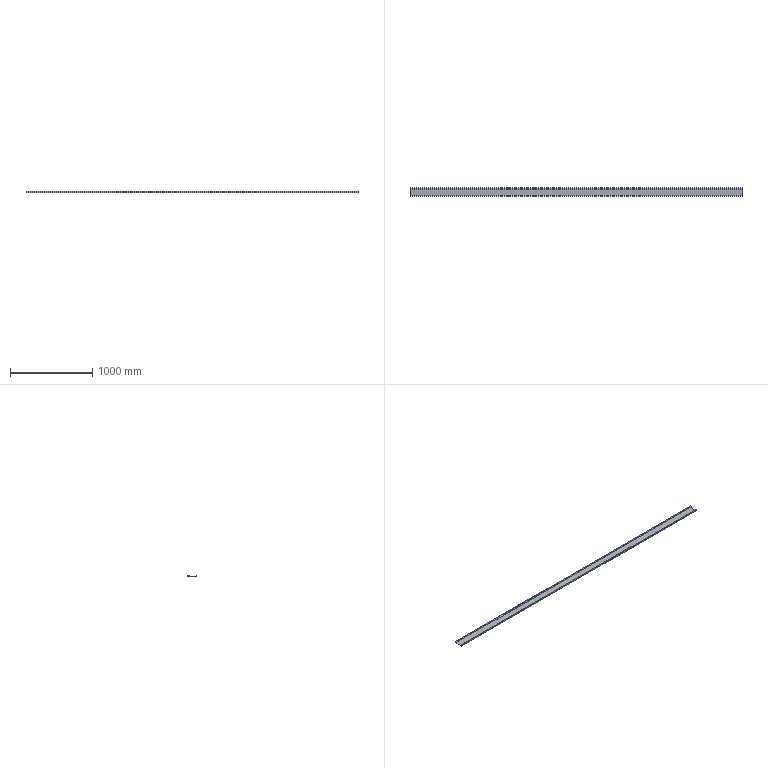Part | STEP file | E3-Electrical cabinet guardrail 1 toe plate | 1 solid | 18 faces | box 4025 x 100 x 20 mm | volume 925227 mm3 | plane 12 | cylinder 6 | commonest cylinder face diameters 2 x3 5 x3
STEP:
#1=CARTESIAN_POINT('',(0.,0.,0.));
#2=DIRECTION('',(0.,0.,1.));
#3=DIRECTION('',(1.,0.,0.));
#4=AXIS2_PLACEMENT_3D('',#1,#2,#3);
#5=CARTESIAN_POINT('',(-2012.5,1.5,2.5));
#6=VERTEX_POINT('',#5);
#7=CARTESIAN_POINT('',(-2012.5,1.5,20.));
#8=VERTEX_POINT('',#7);
#9=CARTESIAN_POINT('',(-2012.5,1.5,2.5));
#10=DIRECTION('',(0.,0.,1.));
#11=VECTOR('',#10,1.);
#12=LINE('',#9,#11);
#13=CARTESIAN_POINT('',(2012.5,1.5,2.5));
#14=DIRECTION('',(0.,-1.,0.));
#15=DIRECTION('',(0.,0.,-1.));
#16=AXIS2_PLACEMENT_3D('',#13,#14,#15);
#17=PLANE('',#16);
#18=CARTESIAN_POINT('',(0.,-4025.));
#19=DIRECTION('',(-1.,0.));
#20=VECTOR('',#19,1.);
#21=LINE('',#18,#20);
#22=(GEOMETRIC_REPRESENTATION_CONTEXT(2)PARAMETRIC_REPRESENTATION_CONTEXT()REPRESENTATION_CONTEXT('',''));
#23=DEFINITIONAL_REPRESENTATION('',(#21),#22);
#24=PCURVE('',#17,#23);
#25=CARTESIAN_POINT('',(-2012.5,2.5,2.5));
#26=DIRECTION('',(-1.,0.,0.));
#27=DIRECTION('',(0.,0.,1.));
#28=AXIS2_PLACEMENT_3D('',#25,#26,#27);
#29=PLANE('',#28);
#30=CARTESIAN_POINT('',(0.,-1.));
#31=DIRECTION('',(1.,0.));
#32=VECTOR('',#31,1.);
#33=LINE('',#30,#32);
#34=(GEOMETRIC_REPRESENTATION_CONTEXT(2)PARAMETRIC_REPRESENTATION_CONTEXT()REPRESENTATION_CONTEXT('',''));
#35=DEFINITIONAL_REPRESENTATION('',(#33),#34);
#36=PCURVE('',#29,#35);
#37=SURFACE_CURVE('',#12,(#24,#36),.PCURVE_S1.);
#38=EDGE_CURVE('',#6,#8,#37,.T.);
#39=ORIENTED_EDGE('',*,*,#38,.T.);
#40=CARTESIAN_POINT('',(2012.5,1.5,20.));
#41=VERTEX_POINT('',#40);
#42=CARTESIAN_POINT('',(2012.5,1.5,20.));
#43=DIRECTION('',(-1.,0.,0.));
#44=VECTOR('',#43,1.);
#45=LINE('',#42,#44);
#46=CARTESIAN_POINT('',(-17.5,0.));
#47=DIRECTION('',(0.,-1.));
#48=VECTOR('',#47,1.);
#49=LINE('',#46,#48);
#50=(GEOMETRIC_REPRESENTATION_CONTEXT(2)PARAMETRIC_REPRESENTATION_CONTEXT()REPRESENTATION_CONTEXT('',''));
#51=DEFINITIONAL_REPRESENTATION('',(#49),#50);
#52=PCURVE('',#17,#51);
#53=CARTESIAN_POINT('',(2012.5,0.,20.));
#54=DIRECTION('',(0.,0.,1.));
#55=DIRECTION('',(1.,0.,0.));
#56=AXIS2_PLACEMENT_3D('',#53,#54,#55);
#57=PLANE('',#56);
#58=CARTESIAN_POINT('',(0.,1.5));
#59=DIRECTION('',(-1.,0.));
#60=VECTOR('',#59,1.);
#61=LINE('',#58,#60);
#62=(GEOMETRIC_REPRESENTATION_CONTEXT(2)PARAMETRIC_REPRESENTATION_CONTEXT()REPRESENTATION_CONTEXT('',''));
#63=DEFINITIONAL_REPRESENTATION('',(#61),#62);
#64=PCURVE('',#57,#63);
#65=SURFACE_CURVE('',#45,(#52,#64),.PCURVE_S1.);
#66=EDGE_CURVE('',#41,#8,#65,.T.);
#67=ORIENTED_EDGE('',*,*,#66,.F.);
#68=CARTESIAN_POINT('',(2012.5,1.5,2.5));
#69=VERTEX_POINT('',#68);
#70=CARTESIAN_POINT('',(2012.5,1.5,2.5));
#71=DIRECTION('',(0.,0.,1.));
#72=VECTOR('',#71,1.);
#73=LINE('',#70,#72);
#74=CARTESIAN_POINT('',(0.,0.));
#75=DIRECTION('',(-1.,0.));
#76=VECTOR('',#75,1.);
#77=LINE('',#74,#76);
#78=(GEOMETRIC_REPRESENTATION_CONTEXT(2)PARAMETRIC_REPRESENTATION_CONTEXT()REPRESENTATION_CONTEXT('',''));
#79=DEFINITIONAL_REPRESENTATION('',(#77),#78);
#80=PCURVE('',#17,#79);
#81=CARTESIAN_POINT('',(2012.5,2.5,2.5));
#82=DIRECTION('',(-1.,0.,0.));
#83=DIRECTION('',(0.,0.,1.));
#84=AXIS2_PLACEMENT_3D('',#81,#82,#83);
#85=PLANE('',#84);
#86=CARTESIAN_POINT('',(0.,-1.));
#87=DIRECTION('',(1.,0.));
#88=VECTOR('',#87,1.);
#89=LINE('',#86,#88);
#90=(GEOMETRIC_REPRESENTATION_CONTEXT(2)PARAMETRIC_REPRESENTATION_CONTEXT()REPRESENTATION_CONTEXT('',''));
#91=DEFINITIONAL_REPRESENTATION('',(#89),#90);
#92=PCURVE('',#85,#91);
#93=SURFACE_CURVE('',#73,(#80,#92),.PCURVE_S1.);
#94=EDGE_CURVE('',#69,#41,#93,.T.);
#95=ORIENTED_EDGE('',*,*,#94,.F.);
#96=CARTESIAN_POINT('',(2012.5,1.5,2.5));
#97=DIRECTION('',(-1.,0.,0.));
#98=VECTOR('',#97,1.);
#99=LINE('',#96,#98);
#100=CARTESIAN_POINT('',(0.,0.));
#101=DIRECTION('',(0.,-1.));
#102=VECTOR('',#101,1.);
#103=LINE('',#100,#102);
#104=(GEOMETRIC_REPRESENTATION_CONTEXT(2)PARAMETRIC_REPRESENTATION_CONTEXT()REPRESENTATION_CONTEXT('',''));
#105=DEFINITIONAL_REPRESENTATION('',(#103),#104);
#106=PCURVE('',#17,#105);
#107=CARTESIAN_POINT('',(2012.5,2.5,2.5));
#108=DIRECTION('',(-1.,0.,0.));
#109=DIRECTION('',(0.,0.,1.));
#110=AXIS2_PLACEMENT_3D('',#107,#108,#109);
#111=CYLINDRICAL_SURFACE('',#110,1.);
#112=CARTESIAN_POINT('',(4.712,0.));
#113=DIRECTION('',(0.,1.));
#114=VECTOR('',#113,1.);
#115=LINE('',#112,#114);
#116=(GEOMETRIC_REPRESENTATION_CONTEXT(2)PARAMETRIC_REPRESENTATION_CONTEXT()REPRESENTATION_CONTEXT('',''));
#117=DEFINITIONAL_REPRESENTATION('',(#115),#116);
#118=PCURVE('',#111,#117);
#119=SURFACE_CURVE('',#99,(#106,#118),.PCURVE_S1.);
#120=EDGE_CURVE('',#69,#6,#119,.T.);
#121=ORIENTED_EDGE('',*,*,#120,.T.);
#122=EDGE_LOOP('',(#39,#67,#95,#121));
#123=FACE_BOUND('',#122,.T.);
#124=ADVANCED_FACE('',(#123),#17,.F.);
#125=CARTESIAN_POINT('',(-2012.5,0.,20.));
#126=VERTEX_POINT('',#125);
#127=CARTESIAN_POINT('',(-2012.5,0.,20.));
#128=DIRECTION('',(0.,1.,0.));
#129=VECTOR('',#128,1.);
#130=LINE('',#127,#129);
#131=CARTESIAN_POINT('',(-4025.,0.));
#132=DIRECTION('',(0.,1.));
#133=VECTOR('',#132,1.);
#134=LINE('',#131,#133);
#135=(GEOMETRIC_REPRESENTATION_CONTEXT(2)PARAMETRIC_REPRESENTATION_CONTEXT()REPRESENTATION_CONTEXT('',''));
#136=DEFINITIONAL_REPRESENTATION('',(#134),#135);
#137=PCURVE('',#57,#136);
#138=CARTESIAN_POINT('',(17.5,-2.5));
#139=DIRECTION('',(0.,1.));
#140=VECTOR('',#139,1.);
#141=LINE('',#138,#140);
#142=(GEOMETRIC_REPRESENTATION_CONTEXT(2)PARAMETRIC_REPRESENTATION_CONTEXT()REPRESENTATION_CONTEXT('',''));
#143=DEFINITIONAL_REPRESENTATION('',(#141),#142);
#144=PCURVE('',#29,#143);
#145=SURFACE_CURVE('',#130,(#137,#144),.PCURVE_S1.);
#146=EDGE_CURVE('',#126,#8,#145,.T.);
#147=ORIENTED_EDGE('',*,*,#146,.F.);
#148=CARTESIAN_POINT('',(2012.5,0.,20.));
#149=VERTEX_POINT('',#148);
#150=CARTESIAN_POINT('',(2012.5,0.,20.));
#151=DIRECTION('',(-1.,0.,0.));
#152=VECTOR('',#151,1.);
#153=LINE('',#150,#152);
#154=CARTESIAN_POINT('',(0.,0.));
#155=DIRECTION('',(-1.,0.));
#156=VECTOR('',#155,1.);
#157=LINE('',#154,#156);
#158=(GEOMETRIC_REPRESENTATION_CONTEXT(2)PARAMETRIC_REPRESENTATION_CONTEXT()REPRESENTATION_CONTEXT('',''));
#159=DEFINITIONAL_REPRESENTATION('',(#157),#158);
#160=PCURVE('',#57,#159);
#161=CARTESIAN_POINT('',(2012.5,0.,2.5));
#162=DIRECTION('',(0.,-1.,0.));
#163=DIRECTION('',(0.,0.,-1.));
#164=AXIS2_PLACEMENT_3D('',#161,#162,#163);
#165=PLANE('',#164);
#166=CARTESIAN_POINT('',(-17.5,0.));
#167=DIRECTION('',(0.,-1.));
#168=VECTOR('',#167,1.);
#169=LINE('',#166,#168);
#170=(GEOMETRIC_REPRESENTATION_CONTEXT(2)PARAMETRIC_REPRESENTATION_CONTEXT()REPRESENTATION_CONTEXT('',''));
#171=DEFINITIONAL_REPRESENTATION('',(#169),#170);
#172=PCURVE('',#165,#171);
#173=SURFACE_CURVE('',#153,(#160,#172),.PCURVE_S1.);
#174=EDGE_CURVE('',#149,#126,#173,.T.);
#175=ORIENTED_EDGE('',*,*,#174,.F.);
#176=CARTESIAN_POINT('',(2012.5,0.,20.));
#177=DIRECTION('',(0.,1.,0.));
#178=VECTOR('',#177,1.);
#179=LINE('',#176,#178);
#180=CARTESIAN_POINT('',(0.,0.));
#181=DIRECTION('',(0.,1.));
#182=VECTOR('',#181,1.);
#183=LINE('',#180,#182);
#184=(GEOMETRIC_REPRESENTATION_CONTEXT(2)PARAMETRIC_REPRESENTATION_CONTEXT()REPRESENTATION_CONTEXT('',''));
#185=DEFINITIONAL_REPRESENTATION('',(#183),#184);
#186=PCURVE('',#57,#185);
#187=CARTESIAN_POINT('',(17.5,-2.5));
#188=DIRECTION('',(0.,1.));
#189=VECTOR('',#188,1.);
#190=LINE('',#187,#189);
#191=(GEOMETRIC_REPRESENTATION_CONTEXT(2)PARAMETRIC_REPRESENTATION_CONTEXT()REPRESENTATION_CONTEXT('',''));
#192=DEFINITIONAL_REPRESENTATION('',(#190),#191);
#193=PCURVE('',#85,#192);
#194=SURFACE_CURVE('',#179,(#186,#193),.PCURVE_S1.);
#195=EDGE_CURVE('',#149,#41,#194,.T.);
#196=ORIENTED_EDGE('',*,*,#195,.T.);
#197=ORIENTED_EDGE('',*,*,#66,.T.);
#198=EDGE_LOOP('',(#147,#175,#196,#197));
#199=FACE_BOUND('',#198,.T.);
#200=ADVANCED_FACE('',(#199),#57,.T.);
#201=CARTESIAN_POINT('',(-2012.5,0.,2.5));
#202=VERTEX_POINT('',#201);
#203=CARTESIAN_POINT('',(-2012.5,0.,2.5));
#204=DIRECTION('',(0.,0.,1.));
#205=VECTOR('',#204,1.);
#206=LINE('',#203,#205);
#207=CARTESIAN_POINT('',(0.,-4025.));
#208=DIRECTION('',(-1.,0.));
#209=VECTOR('',#208,1.);
#210=LINE('',#207,#209);
#211=(GEOMETRIC_REPRESENTATION_CONTEXT(2)PARAMETRIC_REPRESENTATION_CONTEXT()REPRESENTATION_CONTEXT('',''));
#212=DEFINITIONAL_REPRESENTATION('',(#210),#211);
#213=PCURVE('',#165,#212);
#214=CARTESIAN_POINT('',(0.,-2.5));
#215=DIRECTION('',(1.,0.));
#216=VECTOR('',#215,1.);
#217=LINE('',#214,#216);
#218=(GEOMETRIC_REPRESENTATION_CONTEXT(2)PARAMETRIC_REPRESENTATION_CONTEXT()REPRESENTATION_CONTEXT('',''));
#219=DEFINITIONAL_REPRESENTATION('',(#217),#218);
#220=PCURVE('',#29,#219);
#221=SURFACE_CURVE('',#206,(#213,#220),.PCURVE_S1.);
#222=EDGE_CURVE('',#202,#126,#221,.T.);
#223=ORIENTED_EDGE('',*,*,#222,.F.);
#224=CARTESIAN_POINT('',(2012.5,0.,2.5));
#225=VERTEX_POINT('',#224);
#226=CARTESIAN_POINT('',(2012.5,0.,2.5));
#227=DIRECTION('',(-1.,0.,0.));
#228=VECTOR('',#227,1.);
#229=LINE('',#226,#228);
#230=CARTESIAN_POINT('',(0.,0.));
#231=DIRECTION('',(0.,-1.));
#232=VECTOR('',#231,1.);
#233=LINE('',#230,#232);
#234=(GEOMETRIC_REPRESENTATION_CONTEXT(2)PARAMETRIC_REPRESENTATION_CONTEXT()REPRESENTATION_CONTEXT('',''));
#235=DEFINITIONAL_REPRESENTATION('',(#233),#234);
#236=PCURVE('',#165,#235);
#237=CARTESIAN_POINT('',(2012.5,2.5,2.5));
#238=DIRECTION('',(-1.,0.,0.));
#239=DIRECTION('',(0.,0.,1.));
#240=AXIS2_PLACEMENT_3D('',#237,#238,#239);
#241=CYLINDRICAL_SURFACE('',#240,2.5);
#242=CARTESIAN_POINT('',(4.712,0.));
#243=DIRECTION('',(0.,1.));
#244=VECTOR('',#243,1.);
#245=LINE('',#242,#244);
#246=(GEOMETRIC_REPRESENTATION_CONTEXT(2)PARAMETRIC_REPRESENTATION_CONTEXT()REPRESENTATION_CONTEXT('',''));
#247=DEFINITIONAL_REPRESENTATION('',(#245),#246);
#248=PCURVE('',#241,#247);
#249=SURFACE_CURVE('',#229,(#236,#248),.PCURVE_S1.);
#250=EDGE_CURVE('',#225,#202,#249,.T.);
#251=ORIENTED_EDGE('',*,*,#250,.F.);
#252=CARTESIAN_POINT('',(2012.5,0.,2.5));
#253=DIRECTION('',(0.,0.,1.));
#254=VECTOR('',#253,1.);
#255=LINE('',#252,#254);
#256=CARTESIAN_POINT('',(0.,0.));
#257=DIRECTION('',(-1.,0.));
#258=VECTOR('',#257,1.);
#259=LINE('',#256,#258);
#260=(GEOMETRIC_REPRESENTATION_CONTEXT(2)PARAMETRIC_REPRESENTATION_CONTEXT()REPRESENTATION_CONTEXT('',''));
#261=DEFINITIONAL_REPRESENTATION('',(#259),#260);
#262=PCURVE('',#165,#261);
#263=CARTESIAN_POINT('',(0.,-2.5));
#264=DIRECTION('',(1.,0.));
#265=VECTOR('',#264,1.);
#266=LINE('',#263,#265);
#267=(GEOMETRIC_REPRESENTATION_CONTEXT(2)PARAMETRIC_REPRESENTATION_CONTEXT()REPRESENTATION_CONTEXT('',''));
#268=DEFINITIONAL_REPRESENTATION('',(#266),#267);
#269=PCURVE('',#85,#268);
#270=SURFACE_CURVE('',#255,(#262,#269),.PCURVE_S1.);
#271=EDGE_CURVE('',#225,#149,#270,.T.);
#272=ORIENTED_EDGE('',*,*,#271,.T.);
#273=ORIENTED_EDGE('',*,*,#174,.T.);
#274=EDGE_LOOP('',(#223,#251,#272,#273));
#275=FACE_BOUND('',#274,.T.);
#276=ADVANCED_FACE('',(#275),#165,.T.);
#277=CARTESIAN_POINT('',(-2012.5,2.5,0.));
#278=VERTEX_POINT('',#277);
#279=CARTESIAN_POINT('',(-2012.5,2.5,2.5));
#280=DIRECTION('',(-1.,0.,0.));
#281=DIRECTION('',(0.,0.,1.));
#282=AXIS2_PLACEMENT_3D('',#279,#280,#281);
#283=CIRCLE('',#282,2.5);
#284=CARTESIAN_POINT('',(0.,4025.));
#285=DIRECTION('',(1.,0.));
#286=VECTOR('',#285,1.);
#287=LINE('',#284,#286);
#288=(GEOMETRIC_REPRESENTATION_CONTEXT(2)PARAMETRIC_REPRESENTATION_CONTEXT()REPRESENTATION_CONTEXT('',''));
#289=DEFINITIONAL_REPRESENTATION('',(#287),#288);
#290=PCURVE('',#241,#289);
#291=CARTESIAN_POINT('',(0.,0.));
#292=DIRECTION('',(1.,0.));
#293=AXIS2_PLACEMENT_2D('',#291,#292);
#294=CIRCLE('',#293,2.5);
#295=(GEOMETRIC_REPRESENTATION_CONTEXT(2)PARAMETRIC_REPRESENTATION_CONTEXT()REPRESENTATION_CONTEXT('',''));
#296=DEFINITIONAL_REPRESENTATION('',(#294),#295);
#297=PCURVE('',#29,#296);
#298=SURFACE_CURVE('',#283,(#290,#297),.PCURVE_S1.);
#299=EDGE_CURVE('',#278,#202,#298,.T.);
#300=ORIENTED_EDGE('',*,*,#299,.F.);
#301=CARTESIAN_POINT('',(2012.5,2.5,0.));
#302=VERTEX_POINT('',#301);
#303=CARTESIAN_POINT('',(2012.5,2.5,0.));
#304=DIRECTION('',(-1.,0.,0.));
#305=VECTOR('',#304,1.);
#306=LINE('',#303,#305);
#307=CARTESIAN_POINT('',(3.142,0.));
#308=DIRECTION('',(0.,1.));
#309=VECTOR('',#308,1.);
#310=LINE('',#307,#309);
#311=(GEOMETRIC_REPRESENTATION_CONTEXT(2)PARAMETRIC_REPRESENTATION_CONTEXT()REPRESENTATION_CONTEXT('',''));
#312=DEFINITIONAL_REPRESENTATION('',(#310),#311);
#313=PCURVE('',#241,#312);
#314=CARTESIAN_POINT('',(2012.5,2.5,0.));
#315=DIRECTION('',(0.,0.,-1.));
#316=DIRECTION('',(-1.,0.,0.));
#317=AXIS2_PLACEMENT_3D('',#314,#315,#316);
#318=PLANE('',#317);
#319=CARTESIAN_POINT('',(0.,0.));
#320=DIRECTION('',(1.,0.));
#321=VECTOR('',#320,1.);
#322=LINE('',#319,#321);
#323=(GEOMETRIC_REPRESENTATION_CONTEXT(2)PARAMETRIC_REPRESENTATION_CONTEXT()REPRESENTATION_CONTEXT('',''));
#324=DEFINITIONAL_REPRESENTATION('',(#322),#323);
#325=PCURVE('',#318,#324);
#326=SURFACE_CURVE('',#306,(#313,#325),.PCURVE_S1.);
#327=EDGE_CURVE('',#302,#278,#326,.T.);
#328=ORIENTED_EDGE('',*,*,#327,.F.);
#329=CARTESIAN_POINT('',(2012.5,2.5,2.5));
#330=DIRECTION('',(-1.,0.,0.));
#331=DIRECTION('',(0.,0.,1.));
#332=AXIS2_PLACEMENT_3D('',#329,#330,#331);
#333=CIRCLE('',#332,2.5);
#334=CARTESIAN_POINT('',(0.,0.));
#335=DIRECTION('',(1.,0.));
#336=VECTOR('',#335,1.);
#337=LINE('',#334,#336);
#338=(GEOMETRIC_REPRESENTATION_CONTEXT(2)PARAMETRIC_REPRESENTATION_CONTEXT()REPRESENTATION_CONTEXT('',''));
#339=DEFINITIONAL_REPRESENTATION('',(#337),#338);
#340=PCURVE('',#241,#339);
#341=CARTESIAN_POINT('',(0.,0.));
#342=DIRECTION('',(1.,0.));
#343=AXIS2_PLACEMENT_2D('',#341,#342);
#344=CIRCLE('',#343,2.5);
#345=(GEOMETRIC_REPRESENTATION_CONTEXT(2)PARAMETRIC_REPRESENTATION_CONTEXT()REPRESENTATION_CONTEXT('',''));
#346=DEFINITIONAL_REPRESENTATION('',(#344),#345);
#347=PCURVE('',#85,#346);
#348=SURFACE_CURVE('',#333,(#340,#347),.PCURVE_S1.);
#349=EDGE_CURVE('',#302,#225,#348,.T.);
#350=ORIENTED_EDGE('',*,*,#349,.T.);
#351=ORIENTED_EDGE('',*,*,#250,.T.);
#352=EDGE_LOOP('',(#300,#328,#350,#351));
#353=FACE_BOUND('',#352,.T.);
#354=ADVANCED_FACE('',(#353),#241,.T.);
#355=CARTESIAN_POINT('',(-2012.5,97.5,0.));
#356=VERTEX_POINT('',#355);
#357=CARTESIAN_POINT('',(-2012.5,2.5,0.));
#358=DIRECTION('',(0.,-1.,0.));
#359=VECTOR('',#358,1.);
#360=LINE('',#357,#359);
#361=CARTESIAN_POINT('',(4025.,0.));
#362=DIRECTION('',(0.,-1.));
#363=VECTOR('',#362,1.);
#364=LINE('',#361,#363);
#365=(GEOMETRIC_REPRESENTATION_CONTEXT(2)PARAMETRIC_REPRESENTATION_CONTEXT()REPRESENTATION_CONTEXT('',''));
#366=DEFINITIONAL_REPRESENTATION('',(#364),#365);
#367=PCURVE('',#318,#366);
#368=CARTESIAN_POINT('',(-2.5,0.));
#369=DIRECTION('',(0.,-1.));
#370=VECTOR('',#369,1.);
#371=LINE('',#368,#370);
#372=(GEOMETRIC_REPRESENTATION_CONTEXT(2)PARAMETRIC_REPRESENTATION_CONTEXT()REPRESENTATION_CONTEXT('',''));
#373=DEFINITIONAL_REPRESENTATION('',(#371),#372);
#374=PCURVE('',#29,#373);
#375=SURFACE_CURVE('',#360,(#367,#374),.PCURVE_S1.);
#376=EDGE_CURVE('',#356,#278,#375,.T.);
#377=ORIENTED_EDGE('',*,*,#376,.F.);
#378=CARTESIAN_POINT('',(2012.5,97.5,0.));
#379=VERTEX_POINT('',#378);
#380=CARTESIAN_POINT('',(2012.5,97.5,0.));
#381=DIRECTION('',(-1.,0.,0.));
#382=VECTOR('',#381,1.);
#383=LINE('',#380,#382);
#384=CARTESIAN_POINT('',(0.,95.));
#385=DIRECTION('',(1.,0.));
#386=VECTOR('',#385,1.);
#387=LINE('',#384,#386);
#388=(GEOMETRIC_REPRESENTATION_CONTEXT(2)PARAMETRIC_REPRESENTATION_CONTEXT()REPRESENTATION_CONTEXT('',''));
#389=DEFINITIONAL_REPRESENTATION('',(#387),#388);
#390=PCURVE('',#318,#389);
#391=CARTESIAN_POINT('',(2012.5,97.5,2.5));
#392=DIRECTION('',(-1.,0.,0.));
#393=DIRECTION('',(0.,0.,1.));
#394=AXIS2_PLACEMENT_3D('',#391,#392,#393);
#395=CYLINDRICAL_SURFACE('',#394,2.5);
#396=CARTESIAN_POINT('',(3.142,0.));
#397=DIRECTION('',(0.,1.));
#398=VECTOR('',#397,1.);
#399=LINE('',#396,#398);
#400=(GEOMETRIC_REPRESENTATION_CONTEXT(2)PARAMETRIC_REPRESENTATION_CONTEXT()REPRESENTATION_CONTEXT('',''));
#401=DEFINITIONAL_REPRESENTATION('',(#399),#400);
#402=PCURVE('',#395,#401);
#403=SURFACE_CURVE('',#383,(#390,#402),.PCURVE_S1.);
#404=EDGE_CURVE('',#379,#356,#403,.T.);
#405=ORIENTED_EDGE('',*,*,#404,.F.);
#406=CARTESIAN_POINT('',(2012.5,2.5,0.));
#407=DIRECTION('',(0.,-1.,0.));
#408=VECTOR('',#407,1.);
#409=LINE('',#406,#408);
#410=CARTESIAN_POINT('',(0.,0.));
#411=DIRECTION('',(0.,-1.));
#412=VECTOR('',#411,1.);
#413=LINE('',#410,#412);
#414=(GEOMETRIC_REPRESENTATION_CONTEXT(2)PARAMETRIC_REPRESENTATION_CONTEXT()REPRESENTATION_CONTEXT('',''));
#415=DEFINITIONAL_REPRESENTATION('',(#413),#414);
#416=PCURVE('',#318,#415);
#417=CARTESIAN_POINT('',(-2.5,0.));
#418=DIRECTION('',(0.,-1.));
#419=VECTOR('',#418,1.);
#420=LINE('',#417,#419);
#421=(GEOMETRIC_REPRESENTATION_CONTEXT(2)PARAMETRIC_REPRESENTATION_CONTEXT()REPRESENTATION_CONTEXT('',''));
#422=DEFINITIONAL_REPRESENTATION('',(#420),#421);
#423=PCURVE('',#85,#422);
#424=SURFACE_CURVE('',#409,(#416,#423),.PCURVE_S1.);
#425=EDGE_CURVE('',#379,#302,#424,.T.);
#426=ORIENTED_EDGE('',*,*,#425,.T.);
#427=ORIENTED_EDGE('',*,*,#327,.T.);
#428=EDGE_LOOP('',(#377,#405,#426,#427));
#429=FACE_BOUND('',#428,.T.);
#430=ADVANCED_FACE('',(#429),#318,.T.);
#431=CARTESIAN_POINT('',(-2012.5,100.,2.5));
#432=VERTEX_POINT('',#431);
#433=CARTESIAN_POINT('',(-2012.5,97.5,2.5));
#434=DIRECTION('',(-1.,0.,0.));
#435=DIRECTION('',(0.,0.,-1.));
#436=AXIS2_PLACEMENT_3D('',#433,#434,#435);
#437=CIRCLE('',#436,2.5);
#438=CARTESIAN_POINT('',(-3.142,4025.));
#439=DIRECTION('',(1.,0.));
#440=VECTOR('',#439,1.);
#441=LINE('',#438,#440);
#442=(GEOMETRIC_REPRESENTATION_CONTEXT(2)PARAMETRIC_REPRESENTATION_CONTEXT()REPRESENTATION_CONTEXT('',''));
#443=DEFINITIONAL_REPRESENTATION('',(#441),#442);
#444=PCURVE('',#395,#443);
#445=CARTESIAN_POINT('',(0.,95.));
#446=DIRECTION('',(-1.,0.));
#447=AXIS2_PLACEMENT_2D('',#445,#446);
#448=CIRCLE('',#447,2.5);
#449=(GEOMETRIC_REPRESENTATION_CONTEXT(2)PARAMETRIC_REPRESENTATION_CONTEXT()REPRESENTATION_CONTEXT('',''));
#450=DEFINITIONAL_REPRESENTATION('',(#448),#449);
#451=PCURVE('',#29,#450);
#452=SURFACE_CURVE('',#437,(#444,#451),.PCURVE_S1.);
#453=EDGE_CURVE('',#432,#356,#452,.T.);
#454=ORIENTED_EDGE('',*,*,#453,.F.);
#455=CARTESIAN_POINT('',(2012.5,100.,2.5));
#456=VERTEX_POINT('',#455);
#457=CARTESIAN_POINT('',(2012.5,100.,2.5));
#458=DIRECTION('',(-1.,0.,0.));
#459=VECTOR('',#458,1.);
#460=LINE('',#457,#459);
#461=CARTESIAN_POINT('',(1.571,0.));
#462=DIRECTION('',(0.,1.));
#463=VECTOR('',#462,1.);
#464=LINE('',#461,#463);
#465=(GEOMETRIC_REPRESENTATION_CONTEXT(2)PARAMETRIC_REPRESENTATION_CONTEXT()REPRESENTATION_CONTEXT('',''));
#466=DEFINITIONAL_REPRESENTATION('',(#464),#465);
#467=PCURVE('',#395,#466);
#468=CARTESIAN_POINT('',(2012.5,100.,2.5));
#469=DIRECTION('',(0.,1.,0.));
#470=DIRECTION('',(0.,0.,1.));
#471=AXIS2_PLACEMENT_3D('',#468,#469,#470);
#472=PLANE('',#471);
#473=CARTESIAN_POINT('',(0.,0.));
#474=DIRECTION('',(0.,-1.));
#475=VECTOR('',#474,1.);
#476=LINE('',#473,#475);
#477=(GEOMETRIC_REPRESENTATION_CONTEXT(2)PARAMETRIC_REPRESENTATION_CONTEXT()REPRESENTATION_CONTEXT('',''));
#478=DEFINITIONAL_REPRESENTATION('',(#476),#477);
#479=PCURVE('',#472,#478);
#480=SURFACE_CURVE('',#460,(#467,#479),.PCURVE_S1.);
#481=EDGE_CURVE('',#456,#432,#480,.T.);
#482=ORIENTED_EDGE('',*,*,#481,.F.);
#483=CARTESIAN_POINT('',(2012.5,97.5,2.5));
#484=DIRECTION('',(-1.,0.,0.));
#485=DIRECTION('',(0.,0.,-1.));
#486=AXIS2_PLACEMENT_3D('',#483,#484,#485);
#487=CIRCLE('',#486,2.5);
#488=CARTESIAN_POINT('',(-3.142,0.));
#489=DIRECTION('',(1.,0.));
#490=VECTOR('',#489,1.);
#491=LINE('',#488,#490);
#492=(GEOMETRIC_REPRESENTATION_CONTEXT(2)PARAMETRIC_REPRESENTATION_CONTEXT()REPRESENTATION_CONTEXT('',''));
#493=DEFINITIONAL_REPRESENTATION('',(#491),#492);
#494=PCURVE('',#395,#493);
#495=CARTESIAN_POINT('',(0.,95.));
#496=DIRECTION('',(-1.,0.));
#497=AXIS2_PLACEMENT_2D('',#495,#496);
#498=CIRCLE('',#497,2.5);
#499=(GEOMETRIC_REPRESENTATION_CONTEXT(2)PARAMETRIC_REPRESENTATION_CONTEXT()REPRESENTATION_CONTEXT('',''));
#500=DEFINITIONAL_REPRESENTATION('',(#498),#499);
#501=PCURVE('',#85,#500);
#502=SURFACE_CURVE('',#487,(#494,#501),.PCURVE_S1.);
#503=EDGE_CURVE('',#456,#379,#502,.T.);
#504=ORIENTED_EDGE('',*,*,#503,.T.);
#505=ORIENTED_EDGE('',*,*,#404,.T.);
#506=EDGE_LOOP('',(#454,#482,#504,#505));
#507=FACE_BOUND('',#506,.T.);
#508=ADVANCED_FACE('',(#507),#395,.T.);
#509=CARTESIAN_POINT('',(-2012.5,100.,17.5));
#510=VERTEX_POINT('',#509);
#511=CARTESIAN_POINT('',(-2012.5,100.,2.5));
#512=DIRECTION('',(0.,0.,-1.));
#513=VECTOR('',#512,1.);
#514=LINE('',#511,#513);
#515=CARTESIAN_POINT('',(0.,-4025.));
#516=DIRECTION('',(-1.,0.));
#517=VECTOR('',#516,1.);
#518=LINE('',#515,#517);
#519=(GEOMETRIC_REPRESENTATION_CONTEXT(2)PARAMETRIC_REPRESENTATION_CONTEXT()REPRESENTATION_CONTEXT('',''));
#520=DEFINITIONAL_REPRESENTATION('',(#518),#519);
#521=PCURVE('',#472,#520);
#522=CARTESIAN_POINT('',(0.,97.5));
#523=DIRECTION('',(-1.,0.));
#524=VECTOR('',#523,1.);
#525=LINE('',#522,#524);
#526=(GEOMETRIC_REPRESENTATION_CONTEXT(2)PARAMETRIC_REPRESENTATION_CONTEXT()REPRESENTATION_CONTEXT('',''));
#527=DEFINITIONAL_REPRESENTATION('',(#525),#526);
#528=PCURVE('',#29,#527);
#529=SURFACE_CURVE('',#514,(#521,#528),.PCURVE_S1.);
#530=EDGE_CURVE('',#510,#432,#529,.T.);
#531=ORIENTED_EDGE('',*,*,#530,.F.);
#532=CARTESIAN_POINT('',(2012.5,100.,17.5));
#533=VERTEX_POINT('',#532);
#534=CARTESIAN_POINT('',(2012.5,100.,17.5));
#535=DIRECTION('',(-1.,0.,0.));
#536=VECTOR('',#535,1.);
#537=LINE('',#534,#536);
#538=CARTESIAN_POINT('',(15.,0.));
#539=DIRECTION('',(0.,-1.));
#540=VECTOR('',#539,1.);
#541=LINE('',#538,#540);
#542=(GEOMETRIC_REPRESENTATION_CONTEXT(2)PARAMETRIC_REPRESENTATION_CONTEXT()REPRESENTATION_CONTEXT('',''));
#543=DEFINITIONAL_REPRESENTATION('',(#541),#542);
#544=PCURVE('',#472,#543);
#545=CARTESIAN_POINT('',(2012.5,97.5,17.5));
#546=DIRECTION('',(-1.,0.,0.));
#547=DIRECTION('',(0.,0.,1.));
#548=AXIS2_PLACEMENT_3D('',#545,#546,#547);
#549=CYLINDRICAL_SURFACE('',#548,2.5);
#550=CARTESIAN_POINT('',(1.571,0.));
#551=DIRECTION('',(0.,1.));
#552=VECTOR('',#551,1.);
#553=LINE('',#550,#552);
#554=(GEOMETRIC_REPRESENTATION_CONTEXT(2)PARAMETRIC_REPRESENTATION_CONTEXT()REPRESENTATION_CONTEXT('',''));
#555=DEFINITIONAL_REPRESENTATION('',(#553),#554);
#556=PCURVE('',#549,#555);
#557=SURFACE_CURVE('',#537,(#544,#556),.PCURVE_S1.);
#558=EDGE_CURVE('',#533,#510,#557,.T.);
#559=ORIENTED_EDGE('',*,*,#558,.F.);
#560=CARTESIAN_POINT('',(2012.5,100.,2.5));
#561=DIRECTION('',(0.,0.,-1.));
#562=VECTOR('',#561,1.);
#563=LINE('',#560,#562);
#564=CARTESIAN_POINT('',(0.,0.));
#565=DIRECTION('',(-1.,0.));
#566=VECTOR('',#565,1.);
#567=LINE('',#564,#566);
#568=(GEOMETRIC_REPRESENTATION_CONTEXT(2)PARAMETRIC_REPRESENTATION_CONTEXT()REPRESENTATION_CONTEXT('',''));
#569=DEFINITIONAL_REPRESENTATION('',(#567),#568);
#570=PCURVE('',#472,#569);
#571=CARTESIAN_POINT('',(0.,97.5));
#572=DIRECTION('',(-1.,0.));
#573=VECTOR('',#572,1.);
#574=LINE('',#571,#573);
#575=(GEOMETRIC_REPRESENTATION_CONTEXT(2)PARAMETRIC_REPRESENTATION_CONTEXT()REPRESENTATION_CONTEXT('',''));
#576=DEFINITIONAL_REPRESENTATION('',(#574),#575);
#577=PCURVE('',#85,#576);
#578=SURFACE_CURVE('',#563,(#570,#577),.PCURVE_S1.);
#579=EDGE_CURVE('',#533,#456,#578,.T.);
#580=ORIENTED_EDGE('',*,*,#579,.T.);
#581=ORIENTED_EDGE('',*,*,#481,.T.);
#582=EDGE_LOOP('',(#531,#559,#580,#581));
#583=FACE_BOUND('',#582,.T.);
#584=ADVANCED_FACE('',(#583),#472,.T.);
#585=CARTESIAN_POINT('',(-2012.5,97.5,20.));
#586=VERTEX_POINT('',#585);
#587=CARTESIAN_POINT('',(-2012.5,97.5,17.5));
#588=DIRECTION('',(-1.,0.,0.));
#589=DIRECTION('',(0.,0.,-1.));
#590=AXIS2_PLACEMENT_3D('',#587,#588,#589);
#591=CIRCLE('',#590,2.5);
#592=CARTESIAN_POINT('',(-3.142,4025.));
#593=DIRECTION('',(1.,0.));
#594=VECTOR('',#593,1.);
#595=LINE('',#592,#594);
#596=(GEOMETRIC_REPRESENTATION_CONTEXT(2)PARAMETRIC_REPRESENTATION_CONTEXT()REPRESENTATION_CONTEXT('',''));
#597=DEFINITIONAL_REPRESENTATION('',(#595),#596);
#598=PCURVE('',#549,#597);
#599=CARTESIAN_POINT('',(15.,95.));
#600=DIRECTION('',(-1.,0.));
#601=AXIS2_PLACEMENT_2D('',#599,#600);
#602=CIRCLE('',#601,2.5);
#603=(GEOMETRIC_REPRESENTATION_CONTEXT(2)PARAMETRIC_REPRESENTATION_CONTEXT()REPRESENTATION_CONTEXT('',''));
#604=DEFINITIONAL_REPRESENTATION('',(#602),#603);
#605=PCURVE('',#29,#604);
#606=SURFACE_CURVE('',#591,(#598,#605),.PCURVE_S1.);
#607=EDGE_CURVE('',#586,#510,#606,.T.);
#608=ORIENTED_EDGE('',*,*,#607,.F.);
#609=CARTESIAN_POINT('',(2012.5,97.5,20.));
#610=VERTEX_POINT('',#609);
#611=CARTESIAN_POINT('',(2012.5,97.5,20.));
#612=DIRECTION('',(-1.,0.,0.));
#613=VECTOR('',#612,1.);
#614=LINE('',#611,#613);
#615=CARTESIAN_POINT('',(0.,0.));
#616=DIRECTION('',(0.,1.));
#617=VECTOR('',#616,1.);
#618=LINE('',#615,#617);
#619=(GEOMETRIC_REPRESENTATION_CONTEXT(2)PARAMETRIC_REPRESENTATION_CONTEXT()REPRESENTATION_CONTEXT('',''));
#620=DEFINITIONAL_REPRESENTATION('',(#618),#619);
#621=PCURVE('',#549,#620);
#622=CARTESIAN_POINT('',(2012.5,97.5,20.));
#623=DIRECTION('',(0.,0.,1.));
#624=DIRECTION('',(1.,0.,0.));
#625=AXIS2_PLACEMENT_3D('',#622,#623,#624);
#626=PLANE('',#625);
#627=CARTESIAN_POINT('',(0.,0.));
#628=DIRECTION('',(-1.,0.));
#629=VECTOR('',#628,1.);
#630=LINE('',#627,#629);
#631=(GEOMETRIC_REPRESENTATION_CONTEXT(2)PARAMETRIC_REPRESENTATION_CONTEXT()REPRESENTATION_CONTEXT('',''));
#632=DEFINITIONAL_REPRESENTATION('',(#630),#631);
#633=PCURVE('',#626,#632);
#634=SURFACE_CURVE('',#614,(#621,#633),.PCURVE_S1.);
#635=EDGE_CURVE('',#610,#586,#634,.T.);
#636=ORIENTED_EDGE('',*,*,#635,.F.);
#637=CARTESIAN_POINT('',(2012.5,97.5,17.5));
#638=DIRECTION('',(-1.,0.,0.));
#639=DIRECTION('',(0.,0.,-1.));
#640=AXIS2_PLACEMENT_3D('',#637,#638,#639);
#641=CIRCLE('',#640,2.5);
#642=CARTESIAN_POINT('',(-3.142,0.));
#643=DIRECTION('',(1.,0.));
#644=VECTOR('',#643,1.);
#645=LINE('',#642,#644);
#646=(GEOMETRIC_REPRESENTATION_CONTEXT(2)PARAMETRIC_REPRESENTATION_CONTEXT()REPRESENTATION_CONTEXT('',''));
#647=DEFINITIONAL_REPRESENTATION('',(#645),#646);
#648=PCURVE('',#549,#647);
#649=CARTESIAN_POINT('',(15.,95.));
#650=DIRECTION('',(-1.,0.));
#651=AXIS2_PLACEMENT_2D('',#649,#650);
#652=CIRCLE('',#651,2.5);
#653=(GEOMETRIC_REPRESENTATION_CONTEXT(2)PARAMETRIC_REPRESENTATION_CONTEXT()REPRESENTATION_CONTEXT('',''));
#654=DEFINITIONAL_REPRESENTATION('',(#652),#653);
#655=PCURVE('',#85,#654);
#656=SURFACE_CURVE('',#641,(#648,#655),.PCURVE_S1.);
#657=EDGE_CURVE('',#610,#533,#656,.T.);
#658=ORIENTED_EDGE('',*,*,#657,.T.);
#659=ORIENTED_EDGE('',*,*,#558,.T.);
#660=EDGE_LOOP('',(#608,#636,#658,#659));
#661=FACE_BOUND('',#660,.T.);
#662=ADVANCED_FACE('',(#661),#549,.T.);
#663=CARTESIAN_POINT('',(-2012.5,80.,20.));
#664=VERTEX_POINT('',#663);
#665=CARTESIAN_POINT('',(-2012.5,97.5,20.));
#666=DIRECTION('',(0.,1.,0.));
#667=VECTOR('',#666,1.);
#668=LINE('',#665,#667);
#669=CARTESIAN_POINT('',(-4025.,0.));
#670=DIRECTION('',(0.,1.));
#671=VECTOR('',#670,1.);
#672=LINE('',#669,#671);
#673=(GEOMETRIC_REPRESENTATION_CONTEXT(2)PARAMETRIC_REPRESENTATION_CONTEXT()REPRESENTATION_CONTEXT('',''));
#674=DEFINITIONAL_REPRESENTATION('',(#672),#673);
#675=PCURVE('',#626,#674);
#676=CARTESIAN_POINT('',(17.5,95.));
#677=DIRECTION('',(0.,1.));
#678=VECTOR('',#677,1.);
#679=LINE('',#676,#678);
#680=(GEOMETRIC_REPRESENTATION_CONTEXT(2)PARAMETRIC_REPRESENTATION_CONTEXT()REPRESENTATION_CONTEXT('',''));
#681=DEFINITIONAL_REPRESENTATION('',(#679),#680);
#682=PCURVE('',#29,#681);
#683=SURFACE_CURVE('',#668,(#675,#682),.PCURVE_S1.);
#684=EDGE_CURVE('',#664,#586,#683,.T.);
#685=ORIENTED_EDGE('',*,*,#684,.F.);
#686=CARTESIAN_POINT('',(2012.5,80.,20.));
#687=VERTEX_POINT('',#686);
#688=CARTESIAN_POINT('',(2012.5,80.,20.));
#689=DIRECTION('',(-1.,0.,0.));
#690=VECTOR('',#689,1.);
#691=LINE('',#688,#690);
#692=CARTESIAN_POINT('',(0.,-17.5));
#693=DIRECTION('',(-1.,0.));
#694=VECTOR('',#693,1.);
#695=LINE('',#692,#694);
#696=(GEOMETRIC_REPRESENTATION_CONTEXT(2)PARAMETRIC_REPRESENTATION_CONTEXT()REPRESENTATION_CONTEXT('',''));
#697=DEFINITIONAL_REPRESENTATION('',(#695),#696);
#698=PCURVE('',#626,#697);
#699=CARTESIAN_POINT('',(2012.5,80.,18.5));
#700=DIRECTION('',(0.,-1.,0.));
#701=DIRECTION('',(0.,0.,-1.));
#702=AXIS2_PLACEMENT_3D('',#699,#700,#701);
#703=PLANE('',#702);
#704=CARTESIAN_POINT('',(-1.5,0.));
#705=DIRECTION('',(0.,-1.));
#706=VECTOR('',#705,1.);
#707=LINE('',#704,#706);
#708=(GEOMETRIC_REPRESENTATION_CONTEXT(2)PARAMETRIC_REPRESENTATION_CONTEXT()REPRESENTATION_CONTEXT('',''));
#709=DEFINITIONAL_REPRESENTATION('',(#707),#708);
#710=PCURVE('',#703,#709);
#711=SURFACE_CURVE('',#691,(#698,#710),.PCURVE_S1.);
#712=EDGE_CURVE('',#687,#664,#711,.T.);
#713=ORIENTED_EDGE('',*,*,#712,.F.);
#714=CARTESIAN_POINT('',(2012.5,97.5,20.));
#715=DIRECTION('',(0.,1.,0.));
#716=VECTOR('',#715,1.);
#717=LINE('',#714,#716);
#718=CARTESIAN_POINT('',(0.,0.));
#719=DIRECTION('',(0.,1.));
#720=VECTOR('',#719,1.);
#721=LINE('',#718,#720);
#722=(GEOMETRIC_REPRESENTATION_CONTEXT(2)PARAMETRIC_REPRESENTATION_CONTEXT()REPRESENTATION_CONTEXT('',''));
#723=DEFINITIONAL_REPRESENTATION('',(#721),#722);
#724=PCURVE('',#626,#723);
#725=CARTESIAN_POINT('',(17.5,95.));
#726=DIRECTION('',(0.,1.));
#727=VECTOR('',#726,1.);
#728=LINE('',#725,#727);
#729=(GEOMETRIC_REPRESENTATION_CONTEXT(2)PARAMETRIC_REPRESENTATION_CONTEXT()REPRESENTATION_CONTEXT('',''));
#730=DEFINITIONAL_REPRESENTATION('',(#728),#729);
#731=PCURVE('',#85,#730);
#732=SURFACE_CURVE('',#717,(#724,#731),.PCURVE_S1.);
#733=EDGE_CURVE('',#687,#610,#732,.T.);
#734=ORIENTED_EDGE('',*,*,#733,.T.);
#735=ORIENTED_EDGE('',*,*,#635,.T.);
#736=EDGE_LOOP('',(#685,#713,#734,#735));
#737=FACE_BOUND('',#736,.T.);
#738=ADVANCED_FACE('',(#737),#626,.T.);
#739=CARTESIAN_POINT('',(-2012.5,80.,18.5));
#740=VERTEX_POINT('',#739);
#741=CARTESIAN_POINT('',(-2012.5,80.,18.5));
#742=DIRECTION('',(0.,0.,1.));
#743=VECTOR('',#742,1.);
#744=LINE('',#741,#743);
#745=CARTESIAN_POINT('',(0.,-4025.));
#746=DIRECTION('',(-1.,0.));
#747=VECTOR('',#746,1.);
#748=LINE('',#745,#747);
#749=(GEOMETRIC_REPRESENTATION_CONTEXT(2)PARAMETRIC_REPRESENTATION_CONTEXT()REPRESENTATION_CONTEXT('',''));
#750=DEFINITIONAL_REPRESENTATION('',(#748),#749);
#751=PCURVE('',#703,#750);
#752=CARTESIAN_POINT('',(16.,77.5));
#753=DIRECTION('',(1.,0.));
#754=VECTOR('',#753,1.);
#755=LINE('',#752,#754);
#756=(GEOMETRIC_REPRESENTATION_CONTEXT(2)PARAMETRIC_REPRESENTATION_CONTEXT()REPRESENTATION_CONTEXT('',''));
#757=DEFINITIONAL_REPRESENTATION('',(#755),#756);
#758=PCURVE('',#29,#757);
#759=SURFACE_CURVE('',#744,(#751,#758),.PCURVE_S1.);
#760=EDGE_CURVE('',#740,#664,#759,.T.);
#761=ORIENTED_EDGE('',*,*,#760,.F.);
#762=CARTESIAN_POINT('',(2012.5,80.,18.5));
#763=VERTEX_POINT('',#762);
#764=CARTESIAN_POINT('',(2012.5,80.,18.5));
#765=DIRECTION('',(-1.,0.,0.));
#766=VECTOR('',#765,1.);
#767=LINE('',#764,#766);
#768=CARTESIAN_POINT('',(0.,0.));
#769=DIRECTION('',(0.,-1.));
#770=VECTOR('',#769,1.);
#771=LINE('',#768,#770);
#772=(GEOMETRIC_REPRESENTATION_CONTEXT(2)PARAMETRIC_REPRESENTATION_CONTEXT()REPRESENTATION_CONTEXT('',''));
#773=DEFINITIONAL_REPRESENTATION('',(#771),#772);
#774=PCURVE('',#703,#773);
#775=CARTESIAN_POINT('',(2012.5,97.5,18.5));
#776=DIRECTION('',(0.,0.,1.));
#777=DIRECTION('',(1.,0.,0.));
#778=AXIS2_PLACEMENT_3D('',#775,#776,#777);
#779=PLANE('',#778);
#780=CARTESIAN_POINT('',(0.,-17.5));
#781=DIRECTION('',(-1.,0.));
#782=VECTOR('',#781,1.);
#783=LINE('',#780,#782);
#784=(GEOMETRIC_REPRESENTATION_CONTEXT(2)PARAMETRIC_REPRESENTATION_CONTEXT()REPRESENTATION_CONTEXT('',''));
#785=DEFINITIONAL_REPRESENTATION('',(#783),#784);
#786=PCURVE('',#779,#785);
#787=SURFACE_CURVE('',#767,(#774,#786),.PCURVE_S1.);
#788=EDGE_CURVE('',#763,#740,#787,.T.);
#789=ORIENTED_EDGE('',*,*,#788,.F.);
#790=CARTESIAN_POINT('',(2012.5,80.,18.5));
#791=DIRECTION('',(0.,0.,1.));
#792=VECTOR('',#791,1.);
#793=LINE('',#790,#792);
#794=CARTESIAN_POINT('',(0.,0.));
#795=DIRECTION('',(-1.,0.));
#796=VECTOR('',#795,1.);
#797=LINE('',#794,#796);
#798=(GEOMETRIC_REPRESENTATION_CONTEXT(2)PARAMETRIC_REPRESENTATION_CONTEXT()REPRESENTATION_CONTEXT('',''));
#799=DEFINITIONAL_REPRESENTATION('',(#797),#798);
#800=PCURVE('',#703,#799);
#801=CARTESIAN_POINT('',(16.,77.5));
#802=DIRECTION('',(1.,0.));
#803=VECTOR('',#802,1.);
#804=LINE('',#801,#803);
#805=(GEOMETRIC_REPRESENTATION_CONTEXT(2)PARAMETRIC_REPRESENTATION_CONTEXT()REPRESENTATION_CONTEXT('',''));
#806=DEFINITIONAL_REPRESENTATION('',(#804),#805);
#807=PCURVE('',#85,#806);
#808=SURFACE_CURVE('',#793,(#800,#807),.PCURVE_S1.);
#809=EDGE_CURVE('',#763,#687,#808,.T.);
#810=ORIENTED_EDGE('',*,*,#809,.T.);
#811=ORIENTED_EDGE('',*,*,#712,.T.);
#812=EDGE_LOOP('',(#761,#789,#810,#811));
#813=FACE_BOUND('',#812,.T.);
#814=ADVANCED_FACE('',(#813),#703,.T.);
#815=CARTESIAN_POINT('',(-2012.5,97.5,18.5));
#816=VERTEX_POINT('',#815);
#817=CARTESIAN_POINT('',(-2012.5,97.5,18.5));
#818=DIRECTION('',(0.,1.,0.));
#819=VECTOR('',#818,1.);
#820=LINE('',#817,#819);
#821=CARTESIAN_POINT('',(-4025.,0.));
#822=DIRECTION('',(0.,1.));
#823=VECTOR('',#822,1.);
#824=LINE('',#821,#823);
#825=(GEOMETRIC_REPRESENTATION_CONTEXT(2)PARAMETRIC_REPRESENTATION_CONTEXT()REPRESENTATION_CONTEXT('',''));
#826=DEFINITIONAL_REPRESENTATION('',(#824),#825);
#827=PCURVE('',#779,#826);
#828=CARTESIAN_POINT('',(16.,95.));
#829=DIRECTION('',(0.,1.));
#830=VECTOR('',#829,1.);
#831=LINE('',#828,#830);
#832=(GEOMETRIC_REPRESENTATION_CONTEXT(2)PARAMETRIC_REPRESENTATION_CONTEXT()REPRESENTATION_CONTEXT('',''));
#833=DEFINITIONAL_REPRESENTATION('',(#831),#832);
#834=PCURVE('',#29,#833);
#835=SURFACE_CURVE('',#820,(#827,#834),.PCURVE_S1.);
#836=EDGE_CURVE('',#740,#816,#835,.T.);
#837=ORIENTED_EDGE('',*,*,#836,.T.);
#838=CARTESIAN_POINT('',(2012.5,97.5,18.5));
#839=VERTEX_POINT('',#838);
#840=CARTESIAN_POINT('',(2012.5,97.5,18.5));
#841=DIRECTION('',(-1.,0.,0.));
#842=VECTOR('',#841,1.);
#843=LINE('',#840,#842);
#844=CARTESIAN_POINT('',(0.,0.));
#845=DIRECTION('',(-1.,0.));
#846=VECTOR('',#845,1.);
#847=LINE('',#844,#846);
#848=(GEOMETRIC_REPRESENTATION_CONTEXT(2)PARAMETRIC_REPRESENTATION_CONTEXT()REPRESENTATION_CONTEXT('',''));
#849=DEFINITIONAL_REPRESENTATION('',(#847),#848);
#850=PCURVE('',#779,#849);
#851=CARTESIAN_POINT('',(2012.5,97.5,17.5));
#852=DIRECTION('',(-1.,0.,0.));
#853=DIRECTION('',(0.,0.,1.));
#854=AXIS2_PLACEMENT_3D('',#851,#852,#853);
#855=CYLINDRICAL_SURFACE('',#854,1.);
#856=CARTESIAN_POINT('',(0.,0.));
#857=DIRECTION('',(0.,1.));
#858=VECTOR('',#857,1.);
#859=LINE('',#856,#858);
#860=(GEOMETRIC_REPRESENTATION_CONTEXT(2)PARAMETRIC_REPRESENTATION_CONTEXT()REPRESENTATION_CONTEXT('',''));
#861=DEFINITIONAL_REPRESENTATION('',(#859),#860);
#862=PCURVE('',#855,#861);
#863=SURFACE_CURVE('',#843,(#850,#862),.PCURVE_S1.);
#864=EDGE_CURVE('',#839,#816,#863,.T.);
#865=ORIENTED_EDGE('',*,*,#864,.F.);
#866=CARTESIAN_POINT('',(2012.5,97.5,18.5));
#867=DIRECTION('',(0.,1.,0.));
#868=VECTOR('',#867,1.);
#869=LINE('',#866,#868);
#870=CARTESIAN_POINT('',(0.,0.));
#871=DIRECTION('',(0.,1.));
#872=VECTOR('',#871,1.);
#873=LINE('',#870,#872);
#874=(GEOMETRIC_REPRESENTATION_CONTEXT(2)PARAMETRIC_REPRESENTATION_CONTEXT()REPRESENTATION_CONTEXT('',''));
#875=DEFINITIONAL_REPRESENTATION('',(#873),#874);
#876=PCURVE('',#779,#875);
#877=CARTESIAN_POINT('',(16.,95.));
#878=DIRECTION('',(0.,1.));
#879=VECTOR('',#878,1.);
#880=LINE('',#877,#879);
#881=(GEOMETRIC_REPRESENTATION_CONTEXT(2)PARAMETRIC_REPRESENTATION_CONTEXT()REPRESENTATION_CONTEXT('',''));
#882=DEFINITIONAL_REPRESENTATION('',(#880),#881);
#883=PCURVE('',#85,#882);
#884=SURFACE_CURVE('',#869,(#876,#883),.PCURVE_S1.);
#885=EDGE_CURVE('',#763,#839,#884,.T.);
#886=ORIENTED_EDGE('',*,*,#885,.F.);
#887=ORIENTED_EDGE('',*,*,#788,.T.);
#888=EDGE_LOOP('',(#837,#865,#886,#887));
#889=FACE_BOUND('',#888,.T.);
#890=ADVANCED_FACE('',(#889),#779,.F.);
#891=ORIENTED_EDGE('',*,*,#864,.F.);
#892=CARTESIAN_POINT('',(2012.5,98.5,17.5));
#893=VERTEX_POINT('',#892);
#894=CARTESIAN_POINT('',(2012.5,97.5,17.5));
#895=DIRECTION('',(-1.,0.,0.));
#896=DIRECTION('',(0.,0.,-1.));
#897=AXIS2_PLACEMENT_3D('',#894,#895,#896);
#898=CIRCLE('',#897,1.);
#899=CARTESIAN_POINT('',(-3.142,0.));
#900=DIRECTION('',(1.,0.));
#901=VECTOR('',#900,1.);
#902=LINE('',#899,#901);
#903=(GEOMETRIC_REPRESENTATION_CONTEXT(2)PARAMETRIC_REPRESENTATION_CONTEXT()REPRESENTATION_CONTEXT('',''));
#904=DEFINITIONAL_REPRESENTATION('',(#902),#903);
#905=PCURVE('',#855,#904);
#906=CARTESIAN_POINT('',(15.,95.));
#907=DIRECTION('',(-1.,0.));
#908=AXIS2_PLACEMENT_2D('',#906,#907);
#909=CIRCLE('',#908,1.);
#910=(GEOMETRIC_REPRESENTATION_CONTEXT(2)PARAMETRIC_REPRESENTATION_CONTEXT()REPRESENTATION_CONTEXT('',''));
#911=DEFINITIONAL_REPRESENTATION('',(#909),#910);
#912=PCURVE('',#85,#911);
#913=SURFACE_CURVE('',#898,(#905,#912),.PCURVE_S1.);
#914=EDGE_CURVE('',#839,#893,#913,.T.);
#915=ORIENTED_EDGE('',*,*,#914,.T.);
#916=CARTESIAN_POINT('',(-2012.5,98.5,17.5));
#917=VERTEX_POINT('',#916);
#918=CARTESIAN_POINT('',(2012.5,98.5,17.5));
#919=DIRECTION('',(-1.,0.,0.));
#920=VECTOR('',#919,1.);
#921=LINE('',#918,#920);
#922=CARTESIAN_POINT('',(1.571,0.));
#923=DIRECTION('',(0.,1.));
#924=VECTOR('',#923,1.);
#925=LINE('',#922,#924);
#926=(GEOMETRIC_REPRESENTATION_CONTEXT(2)PARAMETRIC_REPRESENTATION_CONTEXT()REPRESENTATION_CONTEXT('',''));
#927=DEFINITIONAL_REPRESENTATION('',(#925),#926);
#928=PCURVE('',#855,#927);
#929=CARTESIAN_POINT('',(2012.5,98.5,2.5));
#930=DIRECTION('',(0.,1.,0.));
#931=DIRECTION('',(0.,0.,1.));
#932=AXIS2_PLACEMENT_3D('',#929,#930,#931);
#933=PLANE('',#932);
#934=CARTESIAN_POINT('',(15.,0.));
#935=DIRECTION('',(0.,-1.));
#936=VECTOR('',#935,1.);
#937=LINE('',#934,#936);
#938=(GEOMETRIC_REPRESENTATION_CONTEXT(2)PARAMETRIC_REPRESENTATION_CONTEXT()REPRESENTATION_CONTEXT('',''));
#939=DEFINITIONAL_REPRESENTATION('',(#937),#938);
#940=PCURVE('',#933,#939);
#941=SURFACE_CURVE('',#921,(#928,#940),.PCURVE_S1.);
#942=EDGE_CURVE('',#893,#917,#941,.T.);
#943=ORIENTED_EDGE('',*,*,#942,.T.);
#944=CARTESIAN_POINT('',(-2012.5,97.5,17.5));
#945=DIRECTION('',(-1.,0.,0.));
#946=DIRECTION('',(0.,0.,-1.));
#947=AXIS2_PLACEMENT_3D('',#944,#945,#946);
#948=CIRCLE('',#947,1.);
#949=CARTESIAN_POINT('',(-3.142,4025.));
#950=DIRECTION('',(1.,0.));
#951=VECTOR('',#950,1.);
#952=LINE('',#949,#951);
#953=(GEOMETRIC_REPRESENTATION_CONTEXT(2)PARAMETRIC_REPRESENTATION_CONTEXT()REPRESENTATION_CONTEXT('',''));
#954=DEFINITIONAL_REPRESENTATION('',(#952),#953);
#955=PCURVE('',#855,#954);
#956=CARTESIAN_POINT('',(15.,95.));
#957=DIRECTION('',(-1.,0.));
#958=AXIS2_PLACEMENT_2D('',#956,#957);
#959=CIRCLE('',#958,1.);
#960=(GEOMETRIC_REPRESENTATION_CONTEXT(2)PARAMETRIC_REPRESENTATION_CONTEXT()REPRESENTATION_CONTEXT('',''));
#961=DEFINITIONAL_REPRESENTATION('',(#959),#960);
#962=PCURVE('',#29,#961);
#963=SURFACE_CURVE('',#948,(#955,#962),.PCURVE_S1.);
#964=EDGE_CURVE('',#816,#917,#963,.T.);
#965=ORIENTED_EDGE('',*,*,#964,.F.);
#966=EDGE_LOOP('',(#891,#915,#943,#965));
#967=FACE_BOUND('',#966,.F.);
#968=ADVANCED_FACE('',(#967),#855,.F.);
#969=CARTESIAN_POINT('',(-2012.5,98.5,2.5));
#970=VERTEX_POINT('',#969);
#971=CARTESIAN_POINT('',(-2012.5,98.5,2.5));
#972=DIRECTION('',(0.,0.,-1.));
#973=VECTOR('',#972,1.);
#974=LINE('',#971,#973);
#975=CARTESIAN_POINT('',(0.,-4025.));
#976=DIRECTION('',(-1.,0.));
#977=VECTOR('',#976,1.);
#978=LINE('',#975,#977);
#979=(GEOMETRIC_REPRESENTATION_CONTEXT(2)PARAMETRIC_REPRESENTATION_CONTEXT()REPRESENTATION_CONTEXT('',''));
#980=DEFINITIONAL_REPRESENTATION('',(#978),#979);
#981=PCURVE('',#933,#980);
#982=CARTESIAN_POINT('',(0.,96.));
#983=DIRECTION('',(-1.,0.));
#984=VECTOR('',#983,1.);
#985=LINE('',#982,#984);
#986=(GEOMETRIC_REPRESENTATION_CONTEXT(2)PARAMETRIC_REPRESENTATION_CONTEXT()REPRESENTATION_CONTEXT('',''));
#987=DEFINITIONAL_REPRESENTATION('',(#985),#986);
#988=PCURVE('',#29,#987);
#989=SURFACE_CURVE('',#974,(#981,#988),.PCURVE_S1.);
#990=EDGE_CURVE('',#917,#970,#989,.T.);
#991=ORIENTED_EDGE('',*,*,#990,.T.);
#992=CARTESIAN_POINT('',(2012.5,98.5,2.5));
#993=VERTEX_POINT('',#992);
#994=CARTESIAN_POINT('',(2012.5,98.5,2.5));
#995=DIRECTION('',(-1.,0.,0.));
#996=VECTOR('',#995,1.);
#997=LINE('',#994,#996);
#998=CARTESIAN_POINT('',(0.,0.));
#999=DIRECTION('',(0.,-1.));
#1000=VECTOR('',#999,1.);
#1001=LINE('',#998,#1000);
#1002=(GEOMETRIC_REPRESENTATION_CONTEXT(2)PARAMETRIC_REPRESENTATION_CONTEXT()REPRESENTATION_CONTEXT('',''));
#1003=DEFINITIONAL_REPRESENTATION('',(#1001),#1002);
#1004=PCURVE('',#933,#1003);
#1005=CARTESIAN_POINT('',(2012.5,97.5,2.5));
#1006=DIRECTION('',(-1.,0.,0.));
#1007=DIRECTION('',(0.,0.,1.));
#1008=AXIS2_PLACEMENT_3D('',#1005,#1006,#1007);
#1009=CYLINDRICAL_SURFACE('',#1008,1.);
#1010=CARTESIAN_POINT('',(1.571,0.));
#1011=DIRECTION('',(0.,1.));
#1012=VECTOR('',#1011,1.);
#1013=LINE('',#1010,#1012);
#1014=(GEOMETRIC_REPRESENTATION_CONTEXT(2)PARAMETRIC_REPRESENTATION_CONTEXT()REPRESENTATION_CONTEXT('',''));
#1015=DEFINITIONAL_REPRESENTATION('',(#1013),#1014);
#1016=PCURVE('',#1009,#1015);
#1017=SURFACE_CURVE('',#997,(#1004,#1016),.PCURVE_S1.);
#1018=EDGE_CURVE('',#993,#970,#1017,.T.);
#1019=ORIENTED_EDGE('',*,*,#1018,.F.);
#1020=CARTESIAN_POINT('',(2012.5,98.5,2.5));
#1021=DIRECTION('',(0.,0.,-1.));
#1022=VECTOR('',#1021,1.);
#1023=LINE('',#1020,#1022);
#1024=CARTESIAN_POINT('',(0.,0.));
#1025=DIRECTION('',(-1.,0.));
#1026=VECTOR('',#1025,1.);
#1027=LINE('',#1024,#1026);
#1028=(GEOMETRIC_REPRESENTATION_CONTEXT(2)PARAMETRIC_REPRESENTATION_CONTEXT()REPRESENTATION_CONTEXT('',''));
#1029=DEFINITIONAL_REPRESENTATION('',(#1027),#1028);
#1030=PCURVE('',#933,#1029);
#1031=CARTESIAN_POINT('',(0.,96.));
#1032=DIRECTION('',(-1.,0.));
#1033=VECTOR('',#1032,1.);
#1034=LINE('',#1031,#1033);
#1035=(GEOMETRIC_REPRESENTATION_CONTEXT(2)PARAMETRIC_REPRESENTATION_CONTEXT()REPRESENTATION_CONTEXT('',''));
#1036=DEFINITIONAL_REPRESENTATION('',(#1034),#1035);
#1037=PCURVE('',#85,#1036);
#1038=SURFACE_CURVE('',#1023,(#1030,#1037),.PCURVE_S1.);
#1039=EDGE_CURVE('',#893,#993,#1038,.T.);
#1040=ORIENTED_EDGE('',*,*,#1039,.F.);
#1041=ORIENTED_EDGE('',*,*,#942,.T.);
#1042=EDGE_LOOP('',(#991,#1019,#1040,#1041));
#1043=FACE_BOUND('',#1042,.T.);
#1044=ADVANCED_FACE('',(#1043),#933,.F.);
#1045=ORIENTED_EDGE('',*,*,#1018,.F.);
#1046=CARTESIAN_POINT('',(2012.5,97.5,1.5));
#1047=VERTEX_POINT('',#1046);
#1048=CARTESIAN_POINT('',(2012.5,97.5,2.5));
#1049=DIRECTION('',(-1.,0.,0.));
#1050=DIRECTION('',(0.,0.,-1.));
#1051=AXIS2_PLACEMENT_3D('',#1048,#1049,#1050);
#1052=CIRCLE('',#1051,1.);
#1053=CARTESIAN_POINT('',(-3.142,0.));
#1054=DIRECTION('',(1.,0.));
#1055=VECTOR('',#1054,1.);
#1056=LINE('',#1053,#1055);
#1057=(GEOMETRIC_REPRESENTATION_CONTEXT(2)PARAMETRIC_REPRESENTATION_CONTEXT()REPRESENTATION_CONTEXT('',''));
#1058=DEFINITIONAL_REPRESENTATION('',(#1056),#1057);
#1059=PCURVE('',#1009,#1058);
#1060=CARTESIAN_POINT('',(0.,95.));
#1061=DIRECTION('',(-1.,0.));
#1062=AXIS2_PLACEMENT_2D('',#1060,#1061);
#1063=CIRCLE('',#1062,1.);
#1064=(GEOMETRIC_REPRESENTATION_CONTEXT(2)PARAMETRIC_REPRESENTATION_CONTEXT()REPRESENTATION_CONTEXT('',''));
#1065=DEFINITIONAL_REPRESENTATION('',(#1063),#1064);
#1066=PCURVE('',#85,#1065);
#1067=SURFACE_CURVE('',#1052,(#1059,#1066),.PCURVE_S1.);
#1068=EDGE_CURVE('',#993,#1047,#1067,.T.);
#1069=ORIENTED_EDGE('',*,*,#1068,.T.);
#1070=CARTESIAN_POINT('',(-2012.5,97.5,1.5));
#1071=VERTEX_POINT('',#1070);
#1072=CARTESIAN_POINT('',(2012.5,97.5,1.5));
#1073=DIRECTION('',(-1.,0.,0.));
#1074=VECTOR('',#1073,1.);
#1075=LINE('',#1072,#1074);
#1076=CARTESIAN_POINT('',(3.142,0.));
#1077=DIRECTION('',(0.,1.));
#1078=VECTOR('',#1077,1.);
#1079=LINE('',#1076,#1078);
#1080=(GEOMETRIC_REPRESENTATION_CONTEXT(2)PARAMETRIC_REPRESENTATION_CONTEXT()REPRESENTATION_CONTEXT('',''));
#1081=DEFINITIONAL_REPRESENTATION('',(#1079),#1080);
#1082=PCURVE('',#1009,#1081);
#1083=CARTESIAN_POINT('',(2012.5,2.5,1.5));
#1084=DIRECTION('',(0.,0.,-1.));
#1085=DIRECTION('',(-1.,0.,0.));
#1086=AXIS2_PLACEMENT_3D('',#1083,#1084,#1085);
#1087=PLANE('',#1086);
#1088=CARTESIAN_POINT('',(0.,95.));
#1089=DIRECTION('',(1.,0.));
#1090=VECTOR('',#1089,1.);
#1091=LINE('',#1088,#1090);
#1092=(GEOMETRIC_REPRESENTATION_CONTEXT(2)PARAMETRIC_REPRESENTATION_CONTEXT()REPRESENTATION_CONTEXT('',''));
#1093=DEFINITIONAL_REPRESENTATION('',(#1091),#1092);
#1094=PCURVE('',#1087,#1093);
#1095=SURFACE_CURVE('',#1075,(#1082,#1094),.PCURVE_S1.);
#1096=EDGE_CURVE('',#1047,#1071,#1095,.T.);
#1097=ORIENTED_EDGE('',*,*,#1096,.T.);
#1098=CARTESIAN_POINT('',(-2012.5,97.5,2.5));
#1099=DIRECTION('',(-1.,0.,0.));
#1100=DIRECTION('',(0.,0.,-1.));
#1101=AXIS2_PLACEMENT_3D('',#1098,#1099,#1100);
#1102=CIRCLE('',#1101,1.);
#1103=CARTESIAN_POINT('',(-3.142,4025.));
#1104=DIRECTION('',(1.,0.));
#1105=VECTOR('',#1104,1.);
#1106=LINE('',#1103,#1105);
#1107=(GEOMETRIC_REPRESENTATION_CONTEXT(2)PARAMETRIC_REPRESENTATION_CONTEXT()REPRESENTATION_CONTEXT('',''));
#1108=DEFINITIONAL_REPRESENTATION('',(#1106),#1107);
#1109=PCURVE('',#1009,#1108);
#1110=CARTESIAN_POINT('',(0.,95.));
#1111=DIRECTION('',(-1.,0.));
#1112=AXIS2_PLACEMENT_2D('',#1110,#1111);
#1113=CIRCLE('',#1112,1.);
#1114=(GEOMETRIC_REPRESENTATION_CONTEXT(2)PARAMETRIC_REPRESENTATION_CONTEXT()REPRESENTATION_CONTEXT('',''));
#1115=DEFINITIONAL_REPRESENTATION('',(#1113),#1114);
#1116=PCURVE('',#29,#1115);
#1117=SURFACE_CURVE('',#1102,(#1109,#1116),.PCURVE_S1.);
#1118=EDGE_CURVE('',#970,#1071,#1117,.T.);
#1119=ORIENTED_EDGE('',*,*,#1118,.F.);
#1120=EDGE_LOOP('',(#1045,#1069,#1097,#1119));
#1121=FACE_BOUND('',#1120,.F.);
#1122=ADVANCED_FACE('',(#1121),#1009,.F.);
#1123=CARTESIAN_POINT('',(-2012.5,2.5,1.5));
#1124=VERTEX_POINT('',#1123);
#1125=CARTESIAN_POINT('',(-2012.5,2.5,1.5));
#1126=DIRECTION('',(0.,-1.,0.));
#1127=VECTOR('',#1126,1.);
#1128=LINE('',#1125,#1127);
#1129=CARTESIAN_POINT('',(4025.,0.));
#1130=DIRECTION('',(0.,-1.));
#1131=VECTOR('',#1130,1.);
#1132=LINE('',#1129,#1131);
#1133=(GEOMETRIC_REPRESENTATION_CONTEXT(2)PARAMETRIC_REPRESENTATION_CONTEXT()REPRESENTATION_CONTEXT('',''));
#1134=DEFINITIONAL_REPRESENTATION('',(#1132),#1133);
#1135=PCURVE('',#1087,#1134);
#1136=CARTESIAN_POINT('',(-1.,0.));
#1137=DIRECTION('',(0.,-1.));
#1138=VECTOR('',#1137,1.);
#1139=LINE('',#1136,#1138);
#1140=(GEOMETRIC_REPRESENTATION_CONTEXT(2)PARAMETRIC_REPRESENTATION_CONTEXT()REPRESENTATION_CONTEXT('',''));
#1141=DEFINITIONAL_REPRESENTATION('',(#1139),#1140);
#1142=PCURVE('',#29,#1141);
#1143=SURFACE_CURVE('',#1128,(#1135,#1142),.PCURVE_S1.);
#1144=EDGE_CURVE('',#1071,#1124,#1143,.T.);
#1145=ORIENTED_EDGE('',*,*,#1144,.T.);
#1146=CARTESIAN_POINT('',(2012.5,2.5,1.5));
#1147=VERTEX_POINT('',#1146);
#1148=CARTESIAN_POINT('',(2012.5,2.5,1.5));
#1149=DIRECTION('',(-1.,0.,0.));
#1150=VECTOR('',#1149,1.);
#1151=LINE('',#1148,#1150);
#1152=CARTESIAN_POINT('',(0.,0.));
#1153=DIRECTION('',(1.,0.));
#1154=VECTOR('',#1153,1.);
#1155=LINE('',#1152,#1154);
#1156=(GEOMETRIC_REPRESENTATION_CONTEXT(2)PARAMETRIC_REPRESENTATION_CONTEXT()REPRESENTATION_CONTEXT('',''));
#1157=DEFINITIONAL_REPRESENTATION('',(#1155),#1156);
#1158=PCURVE('',#1087,#1157);
#1159=CARTESIAN_POINT('',(3.142,0.));
#1160=DIRECTION('',(0.,1.));
#1161=VECTOR('',#1160,1.);
#1162=LINE('',#1159,#1161);
#1163=(GEOMETRIC_REPRESENTATION_CONTEXT(2)PARAMETRIC_REPRESENTATION_CONTEXT()REPRESENTATION_CONTEXT('',''));
#1164=DEFINITIONAL_REPRESENTATION('',(#1162),#1163);
#1165=PCURVE('',#111,#1164);
#1166=SURFACE_CURVE('',#1151,(#1158,#1165),.PCURVE_S1.);
#1167=EDGE_CURVE('',#1147,#1124,#1166,.T.);
#1168=ORIENTED_EDGE('',*,*,#1167,.F.);
#1169=CARTESIAN_POINT('',(2012.5,2.5,1.5));
#1170=DIRECTION('',(0.,-1.,0.));
#1171=VECTOR('',#1170,1.);
#1172=LINE('',#1169,#1171);
#1173=CARTESIAN_POINT('',(0.,0.));
#1174=DIRECTION('',(0.,-1.));
#1175=VECTOR('',#1174,1.);
#1176=LINE('',#1173,#1175);
#1177=(GEOMETRIC_REPRESENTATION_CONTEXT(2)PARAMETRIC_REPRESENTATION_CONTEXT()REPRESENTATION_CONTEXT('',''));
#1178=DEFINITIONAL_REPRESENTATION('',(#1176),#1177);
#1179=PCURVE('',#1087,#1178);
#1180=CARTESIAN_POINT('',(-1.,0.));
#1181=DIRECTION('',(0.,-1.));
#1182=VECTOR('',#1181,1.);
#1183=LINE('',#1180,#1182);
#1184=(GEOMETRIC_REPRESENTATION_CONTEXT(2)PARAMETRIC_REPRESENTATION_CONTEXT()REPRESENTATION_CONTEXT('',''));
#1185=DEFINITIONAL_REPRESENTATION('',(#1183),#1184);
#1186=PCURVE('',#85,#1185);
#1187=SURFACE_CURVE('',#1172,(#1179,#1186),.PCURVE_S1.);
#1188=EDGE_CURVE('',#1047,#1147,#1187,.T.);
#1189=ORIENTED_EDGE('',*,*,#1188,.F.);
#1190=ORIENTED_EDGE('',*,*,#1096,.T.);
#1191=EDGE_LOOP('',(#1145,#1168,#1189,#1190));
#1192=FACE_BOUND('',#1191,.T.);
#1193=ADVANCED_FACE('',(#1192),#1087,.F.);
#1194=ORIENTED_EDGE('',*,*,#1167,.F.);
#1195=CARTESIAN_POINT('',(2012.5,2.5,2.5));
#1196=DIRECTION('',(-1.,0.,0.));
#1197=DIRECTION('',(0.,0.,-1.));
#1198=AXIS2_PLACEMENT_3D('',#1195,#1196,#1197);
#1199=CIRCLE('',#1198,1.);
#1200=CARTESIAN_POINT('',(3.142,0.));
#1201=DIRECTION('',(1.,0.));
#1202=VECTOR('',#1201,1.);
#1203=LINE('',#1200,#1202);
#1204=(GEOMETRIC_REPRESENTATION_CONTEXT(2)PARAMETRIC_REPRESENTATION_CONTEXT()REPRESENTATION_CONTEXT('',''));
#1205=DEFINITIONAL_REPRESENTATION('',(#1203),#1204);
#1206=PCURVE('',#111,#1205);
#1207=CARTESIAN_POINT('',(0.,0.));
#1208=DIRECTION('',(-1.,0.));
#1209=AXIS2_PLACEMENT_2D('',#1207,#1208);
#1210=CIRCLE('',#1209,1.);
#1211=(GEOMETRIC_REPRESENTATION_CONTEXT(2)PARAMETRIC_REPRESENTATION_CONTEXT()REPRESENTATION_CONTEXT('',''));
#1212=DEFINITIONAL_REPRESENTATION('',(#1210),#1211);
#1213=PCURVE('',#85,#1212);
#1214=SURFACE_CURVE('',#1199,(#1206,#1213),.PCURVE_S1.);
#1215=EDGE_CURVE('',#1147,#69,#1214,.T.);
#1216=ORIENTED_EDGE('',*,*,#1215,.T.);
#1217=ORIENTED_EDGE('',*,*,#120,.T.);
#1218=CARTESIAN_POINT('',(-2012.5,2.5,2.5));
#1219=DIRECTION('',(-1.,0.,0.));
#1220=DIRECTION('',(0.,0.,-1.));
#1221=AXIS2_PLACEMENT_3D('',#1218,#1219,#1220);
#1222=CIRCLE('',#1221,1.);
#1223=CARTESIAN_POINT('',(3.142,4025.));
#1224=DIRECTION('',(1.,0.));
#1225=VECTOR('',#1224,1.);
#1226=LINE('',#1223,#1225);
#1227=(GEOMETRIC_REPRESENTATION_CONTEXT(2)PARAMETRIC_REPRESENTATION_CONTEXT()REPRESENTATION_CONTEXT('',''));
#1228=DEFINITIONAL_REPRESENTATION('',(#1226),#1227);
#1229=PCURVE('',#111,#1228);
#1230=CARTESIAN_POINT('',(0.,0.));
#1231=DIRECTION('',(-1.,0.));
#1232=AXIS2_PLACEMENT_2D('',#1230,#1231);
#1233=CIRCLE('',#1232,1.);
#1234=(GEOMETRIC_REPRESENTATION_CONTEXT(2)PARAMETRIC_REPRESENTATION_CONTEXT()REPRESENTATION_CONTEXT('',''));
#1235=DEFINITIONAL_REPRESENTATION('',(#1233),#1234);
#1236=PCURVE('',#29,#1235);
#1237=SURFACE_CURVE('',#1222,(#1229,#1236),.PCURVE_S1.);
#1238=EDGE_CURVE('',#1124,#6,#1237,.T.);
#1239=ORIENTED_EDGE('',*,*,#1238,.F.);
#1240=EDGE_LOOP('',(#1194,#1216,#1217,#1239));
#1241=FACE_BOUND('',#1240,.F.);
#1242=ADVANCED_FACE('',(#1241),#111,.F.);
#1243=ORIENTED_EDGE('',*,*,#94,.T.);
#1244=ORIENTED_EDGE('',*,*,#195,.F.);
#1245=ORIENTED_EDGE('',*,*,#271,.F.);
#1246=ORIENTED_EDGE('',*,*,#349,.F.);
#1247=ORIENTED_EDGE('',*,*,#425,.F.);
#1248=ORIENTED_EDGE('',*,*,#503,.F.);
#1249=ORIENTED_EDGE('',*,*,#579,.F.);
#1250=ORIENTED_EDGE('',*,*,#657,.F.);
#1251=ORIENTED_EDGE('',*,*,#733,.F.);
#1252=ORIENTED_EDGE('',*,*,#809,.F.);
#1253=ORIENTED_EDGE('',*,*,#885,.T.);
#1254=ORIENTED_EDGE('',*,*,#914,.T.);
#1255=ORIENTED_EDGE('',*,*,#1039,.T.);
#1256=ORIENTED_EDGE('',*,*,#1068,.T.);
#1257=ORIENTED_EDGE('',*,*,#1188,.T.);
#1258=ORIENTED_EDGE('',*,*,#1215,.T.);
#1259=EDGE_LOOP('',(#1243,#1244,#1245,#1246,#1247,#1248,#1249,#1250,#1251,#1252,#1253,#1254,#1255,#1256,#1257,#1258));
#1260=FACE_BOUND('',#1259,.T.);
#1261=ADVANCED_FACE('',(#1260),#85,.F.);
#1262=ORIENTED_EDGE('',*,*,#38,.F.);
#1263=ORIENTED_EDGE('',*,*,#1238,.F.);
#1264=ORIENTED_EDGE('',*,*,#1144,.F.);
#1265=ORIENTED_EDGE('',*,*,#1118,.F.);
#1266=ORIENTED_EDGE('',*,*,#990,.F.);
#1267=ORIENTED_EDGE('',*,*,#964,.F.);
#1268=ORIENTED_EDGE('',*,*,#836,.F.);
#1269=ORIENTED_EDGE('',*,*,#760,.T.);
#1270=ORIENTED_EDGE('',*,*,#684,.T.);
#1271=ORIENTED_EDGE('',*,*,#607,.T.);
#1272=ORIENTED_EDGE('',*,*,#530,.T.);
#1273=ORIENTED_EDGE('',*,*,#453,.T.);
#1274=ORIENTED_EDGE('',*,*,#376,.T.);
#1275=ORIENTED_EDGE('',*,*,#299,.T.);
#1276=ORIENTED_EDGE('',*,*,#222,.T.);
#1277=ORIENTED_EDGE('',*,*,#146,.T.);
#1278=EDGE_LOOP('',(#1262,#1263,#1264,#1265,#1266,#1267,#1268,#1269,#1270,#1271,#1272,#1273,#1274,#1275,#1276,#1277));
#1279=FACE_BOUND('',#1278,.T.);
#1280=ADVANCED_FACE('',(#1279),#29,.T.);
#1281=CLOSED_SHELL('',(#124,#200,#276,#354,#430,#508,#584,#662,#738,#814,#890,#968,#1044,#1122,#1193,#1242,#1261,#1280));
#1282=MANIFOLD_SOLID_BREP('',#1281);
#1283=(LENGTH_UNIT()NAMED_UNIT(*)SI_UNIT(.MILLI.,.METRE.));
#1284=UNCERTAINTY_MEASURE_WITH_UNIT(LENGTH_MEASURE(0.0000001),#1283,'','');
#1285=(NAMED_UNIT(*)PLANE_ANGLE_UNIT()SI_UNIT($,.RADIAN.));
#1286=(NAMED_UNIT(*)SI_UNIT($,.STERADIAN.)SOLID_ANGLE_UNIT());
#1287=(GEOMETRIC_REPRESENTATION_CONTEXT(3)GLOBAL_UNCERTAINTY_ASSIGNED_CONTEXT((#1284))GLOBAL_UNIT_ASSIGNED_CONTEXT((#1283,#1285,#1286))REPRESENTATION_CONTEXT('',''));
#1288=ADVANCED_BREP_SHAPE_REPRESENTATION('',(#4,#1282),#1287);